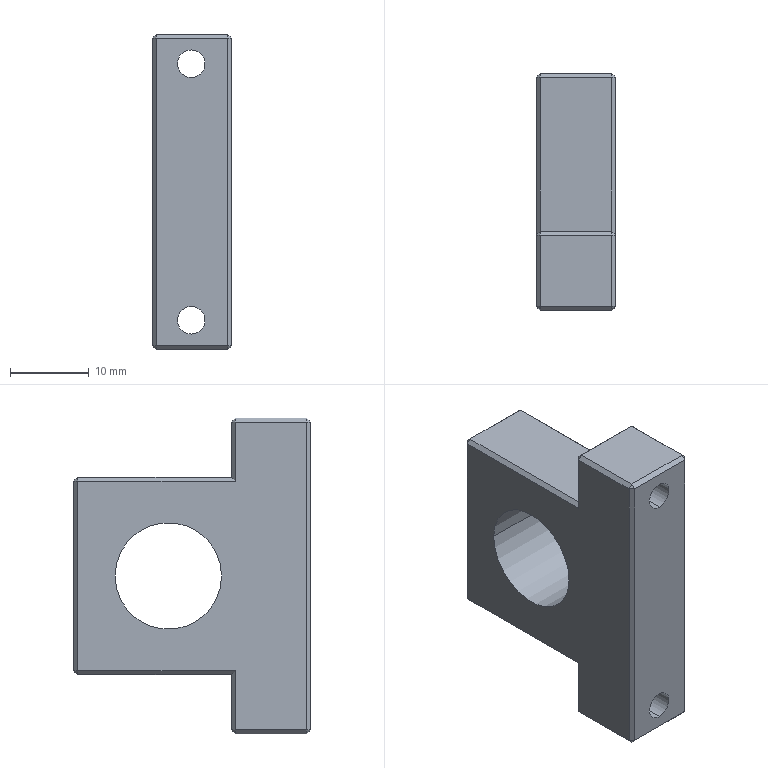Part | STEP file | 06-27 Cutter cylinder fixing block | 1 solid | 50 faces | box 10 x 30 x 40 mm | volume 7335 mm3 | plane 44 | cylinder 6 | commonest cylinder face diameters 3.5 x4 13.5 x2